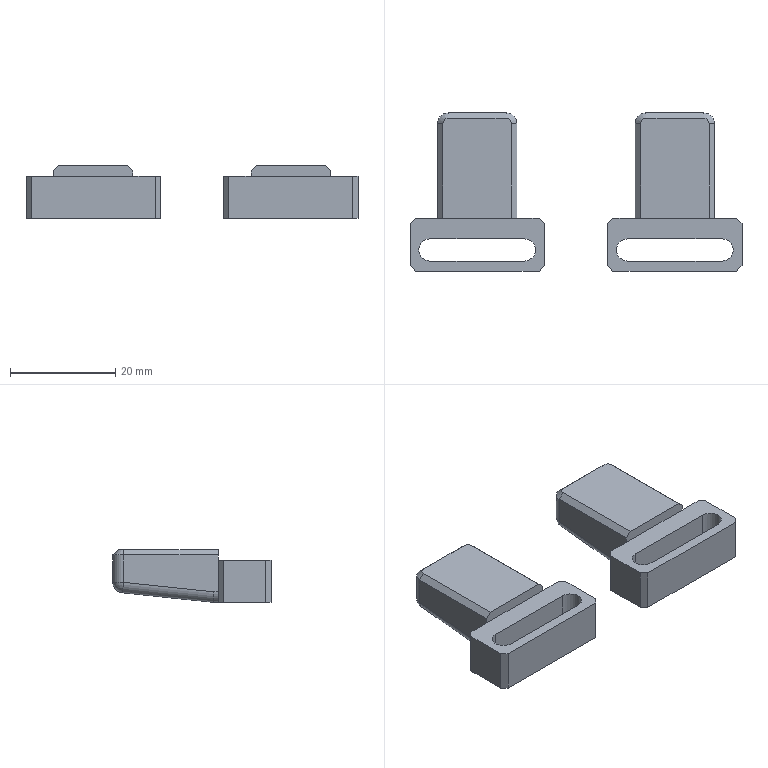NC program | NX | posted with a generic post | part box 63 x 30 x 10 mm
Lines 1610 to 2151 of 2151:
(ZLEVEL_PROFILE_COPY , TOOL : D3)
N3188 T17 M6
N3190 G54
N3192 G17 G0 G90 X-22.132 Y-11.6 B0. C0. S9500 M3
N3194 G43 Z30. H17
N3196 Z-0.5
N3198 G94 G1 X-9.558 Z-1.159 F1000.
N3200 X-9.23 Y-11.356 Z-1.18
N3202 X-9.121 Y-10.962 Z-1.202
N3204 X-9.26 Y-10.604 Z-1.222
N3206 X-9.558 Y-10.4 Z-1.241
N3208 X-27.942 Z-2.204
N3210 X-28.24 Y-10.604 Z-2.223
N3212 X-28.379 Y-10.962 Z-2.243
N3214 X-28.27 Y-11.356 Z-2.265
N3216 X-27.942 Y-11.6 Z-2.286
N3218 X-27.75 Z-2.296
N3220 X-9.75 F1200.
N3222 G3 X-9.15 Y-11. R0.6
N3224 X-9.75 Y-10.4 R0.6
N3226 G1 X-27.75
N3228 G3 X-28.35 Y-11. R0.6
N3230 X-27.75 Y-11.6 R0.6
N3232 G1 X-10.775 Z-2.593
N3234 X-9.75
N3236 G3 X-9.15 Y-11. R0.6
N3238 X-9.75 Y-10.4 R0.6
N3240 G1 X-27.75
N3242 G3 X-28.35 Y-11. R0.6
N3244 X-27.75 Y-11.6 R0.6
N3246 G1 X-10.775 Z-2.889
N3248 X-9.75
N3250 G3 X-9.15 Y-11. R0.6
N3252 X-9.75 Y-10.4 R0.6
N3254 G1 X-27.75
N3256 G3 X-28.35 Y-11. R0.6
N3258 X-27.75 Y-11.6 R0.6
N3260 G1 X-10.775 Z-3.185
N3262 X-9.75
N3264 G3 X-9.15 Y-11. R0.6
N3266 X-9.75 Y-10.4 R0.6
N3268 G1 X-27.75
N3270 G3 X-28.35 Y-11. R0.6
N3272 X-27.75 Y-11.6 R0.6
N3274 G1 X-10.775 Z-3.481
N3276 X-9.75
N3278 G3 X-9.15 Y-11. R0.6
N3280 X-9.75 Y-10.4 R0.6
N3282 G1 X-27.75
N3284 G3 X-28.35 Y-11. R0.6
N3286 X-27.75 Y-11.6 R0.6
N3288 G1 X-10.775 Z-3.778
N3290 X-9.75
N3292 G3 X-9.15 Y-11. R0.6
N3294 X-9.75 Y-10.4 R0.6
N3296 G1 X-27.75
N3298 G3 X-28.35 Y-11. R0.6
N3300 X-27.75 Y-11.6 R0.6
N3302 G1 X-10.775 Z-4.074
N3304 X-9.75
N3306 G3 X-9.15 Y-11. R0.6
N3308 X-9.75 Y-10.4 R0.6
N3310 G1 X-27.75
N3312 G3 X-28.35 Y-11. R0.6
N3314 X-27.75 Y-11.6 R0.6
N3316 G1 X-10.775 Z-4.37
N3318 X-9.75
N3320 G3 X-9.15 Y-11. R0.6
N3322 X-9.75 Y-10.4 R0.6
N3324 G1 X-27.75
N3326 G3 X-28.35 Y-11. R0.6
N3328 X-27.75 Y-11.6 R0.6
N3330 G1 X-10.775 Z-4.667
N3332 X-9.75
N3334 G3 X-9.15 Y-11. R0.6
N3336 X-9.75 Y-10.4 R0.6
N3338 G1 X-27.75
N3340 G3 X-28.35 Y-11. R0.6
N3342 X-27.75 Y-11.6 R0.6
N3344 G1 X-10.775 Z-4.963
N3346 X-9.75
N3348 G3 X-9.15 Y-11. R0.6
N3350 X-9.75 Y-10.4 R0.6
N3352 G1 X-27.75
N3354 G3 X-28.35 Y-11. R0.6
N3356 X-27.75 Y-11.6 R0.6
N3358 G1 X-10.775 Z-5.259
N3360 X-9.75
N3362 G3 X-9.15 Y-11. R0.6
N3364 X-9.75 Y-10.4 R0.6
N3366 G1 X-27.75
N3368 G3 X-28.35 Y-11. R0.6
N3370 X-27.75 Y-11.6 R0.6
N3372 G1 X-10.775 Z-5.556
N3374 X-9.75
N3376 G3 X-9.15 Y-11. R0.6
N3378 X-9.75 Y-10.4 R0.6
N3380 G1 X-27.75
N3382 G3 X-28.35 Y-11. R0.6
N3384 X-27.75 Y-11.6 R0.6
N3386 G1 X-10.775 Z-5.852
N3388 X-9.75
N3390 G3 X-9.15 Y-11. R0.6
N3392 X-9.75 Y-10.4 R0.6
N3394 G1 X-27.75
N3396 G3 X-28.35 Y-11. R0.6
N3398 X-27.75 Y-11.6 R0.6
N3400 G1 X-10.775 Z-6.148
N3402 X-9.75
N3404 G3 X-9.15 Y-11. R0.6
N3406 X-9.75 Y-10.4 R0.6
N3408 G1 X-27.75
N3410 G3 X-28.35 Y-11. R0.6
N3412 X-27.75 Y-11.6 R0.6
N3414 G1 X-10.775 Z-6.444
N3416 X-9.75
N3418 G3 X-9.15 Y-11. R0.6
N3420 X-9.75 Y-10.4 R0.6
N3422 G1 X-27.75
N3424 G3 X-28.35 Y-11. R0.6
N3426 X-27.75 Y-11.6 R0.6
N3428 G1 X-10.775 Z-6.741
N3430 X-9.75
N3432 G3 X-9.15 Y-11. R0.6
N3434 X-9.75 Y-10.4 R0.6
N3436 G1 X-27.75
N3438 G3 X-28.35 Y-11. R0.6
N3440 X-27.75 Y-11.6 R0.6
N3442 G1 X-10.775 Z-7.037
N3444 X-9.75
N3446 G3 X-9.15 Y-11. R0.6
N3448 X-9.75 Y-10.4 R0.6
N3450 G1 X-27.75
N3452 G3 X-28.35 Y-11. R0.6
N3454 X-27.75 Y-11.6 R0.6
N3456 G1 X-10.775 Z-7.333
N3458 X-9.75
N3460 G3 X-9.15 Y-11. R0.6
N3462 X-9.75 Y-10.4 R0.6
N3464 G1 X-27.75
N3466 G3 X-28.35 Y-11. R0.6
N3468 X-27.75 Y-11.6 R0.6
N3470 G1 X-10.775 Z-7.63
N3472 X-9.75
N3474 G3 X-9.15 Y-11. R0.6
N3476 X-9.75 Y-10.4 R0.6
N3478 G1 X-27.75
N3480 G3 X-28.35 Y-11. R0.6
N3482 X-27.75 Y-11.6 R0.6
N3484 G1 X-10.775 Z-7.926
N3486 X-9.75
N3488 G3 X-9.15 Y-11. R0.6
N3490 X-9.75 Y-10.4 R0.6
N3492 G1 X-27.75
N3494 G3 X-28.35 Y-11. R0.6
N3496 X-27.75 Y-11.6 R0.6
N3498 G1 X-10.775 Z-8.222
N3500 X-9.75
N3502 G3 X-9.15 Y-11. R0.6
N3504 X-9.75 Y-10.4 R0.6
N3506 G1 X-27.75
N3508 G3 X-28.35 Y-11. R0.6
N3510 X-27.75 Y-11.6 R0.6
N3512 G1 X-10.775 Z-8.519
N3514 X-9.75
N3516 G3 X-9.15 Y-11. R0.6
N3518 X-9.75 Y-10.4 R0.6
N3520 G1 X-27.75
N3522 G3 X-28.35 Y-11. R0.6
N3524 X-27.75 Y-11.6 R0.6
N3526 G1 X-10.775 Z-8.815
N3528 X-9.75
N3530 G3 X-9.15 Y-11. R0.6
N3532 X-9.75 Y-10.4 R0.6
N3534 G1 X-27.75
N3536 G3 X-28.35 Y-11. R0.6
N3538 X-27.75 Y-11.6 R0.6
N3540 G1 X-10.775 Z-9.111
N3542 X-9.75
N3544 G3 X-9.15 Y-11. R0.6
N3546 X-9.75 Y-10.4 R0.6
N3548 G1 X-27.75
N3550 G3 X-28.35 Y-11. R0.6
N3552 X-27.75 Y-11.6 R0.6
N3554 G1 X-10.775 Z-9.407
N3556 X-9.75
N3558 G3 X-9.15 Y-11. R0.6
N3560 X-9.75 Y-10.4 R0.6
N3562 G1 X-27.75
N3564 G3 X-28.35 Y-11. R0.6
N3566 X-27.75 Y-11.6 R0.6
N3568 G1 X-10.775 Z-9.704
N3570 X-9.75
N3572 G3 X-9.15 Y-11. R0.6
N3574 X-9.75 Y-10.4 R0.6
N3576 G1 X-27.75
N3578 G3 X-28.35 Y-11. R0.6
N3580 X-27.75 Y-11.6 R0.6
N3582 G1 X-10.775 Z-10.
N3584 X-9.75
N3586 G3 X-9.15 Y-11. R0.6
N3588 X-9.75 Y-10.4 R0.6
N3590 G1 X-27.75
N3592 G3 X-28.35 Y-11. R0.6
N3594 X-27.75 Y-11.6 R0.6
N3596 G1 X-10.775
N3598 Z-8.5
N3600 G0 Z30.
N3602 X15.368
N3604 Z-0.5
N3606 G1 X27.942 Z-1.159 F1000.
N3608 X28.27 Y-11.356 Z-1.18
N3610 X28.379 Y-10.962 Z-1.202
N3612 X28.24 Y-10.604 Z-1.222
N3614 X27.942 Y-10.4 Z-1.241
N3616 X9.558 Z-2.204
N3618 X9.26 Y-10.604 Z-2.223
N3620 X9.121 Y-10.962 Z-2.243
N3622 X9.23 Y-11.356 Z-2.265
N3624 X9.558 Y-11.6 Z-2.286
N3626 X9.75 Z-2.296
N3628 X27.75 F1200.
N3630 G3 X28.35 Y-11. R0.6
N3632 X27.75 Y-10.4 R0.6
N3634 G1 X9.75
N3636 G3 X9.15 Y-11. R0.6
N3638 X9.75 Y-11.6 R0.6
N3640 G1 X26.725 Z-2.593
N3642 X27.75
N3644 G3 X28.35 Y-11. R0.6
N3646 X27.75 Y-10.4 R0.6
N3648 G1 X9.75
N3650 G3 X9.15 Y-11. R0.6
N3652 X9.75 Y-11.6 R0.6
N3654 G1 X26.725 Z-2.889
N3656 X27.75
N3658 G3 X28.35 Y-11. R0.6
N3660 X27.75 Y-10.4 R0.6
N3662 G1 X9.75
N3664 G3 X9.15 Y-11. R0.6
N3666 X9.75 Y-11.6 R0.6
N3668 G1 X26.725 Z-3.185
N3670 X27.75
N3672 G3 X28.35 Y-11. R0.6
N3674 X27.75 Y-10.4 R0.6
N3676 G1 X9.75
N3678 G3 X9.15 Y-11. R0.6
N3680 X9.75 Y-11.6 R0.6
N3682 G1 X26.725 Z-3.481
N3684 X27.75
N3686 G3 X28.35 Y-11. R0.6
N3688 X27.75 Y-10.4 R0.6
N3690 G1 X9.75
N3692 G3 X9.15 Y-11. R0.6
N3694 X9.75 Y-11.6 R0.6
N3696 G1 X26.725 Z-3.778
N3698 X27.75
N3700 G3 X28.35 Y-11. R0.6
N3702 X27.75 Y-10.4 R0.6
N3704 G1 X9.75
N3706 G3 X9.15 Y-11. R0.6
N3708 X9.75 Y-11.6 R0.6
N3710 G1 X26.725 Z-4.074
N3712 X27.75
N3714 G3 X28.35 Y-11. R0.6
N3716 X27.75 Y-10.4 R0.6
N3718 G1 X9.75
N3720 G3 X9.15 Y-11. R0.6
N3722 X9.75 Y-11.6 R0.6
N3724 G1 X26.725 Z-4.37
N3726 X27.75
N3728 G3 X28.35 Y-11. R0.6
N3730 X27.75 Y-10.4 R0.6
N3732 G1 X9.75
N3734 G3 X9.15 Y-11. R0.6
N3736 X9.75 Y-11.6 R0.6
N3738 G1 X26.725 Z-4.667
N3740 X27.75
N3742 G3 X28.35 Y-11. R0.6
N3744 X27.75 Y-10.4 R0.6
N3746 G1 X9.75
N3748 G3 X9.15 Y-11. R0.6
N3750 X9.75 Y-11.6 R0.6
N3752 G1 X26.725 Z-4.963
N3754 X27.75
N3756 G3 X28.35 Y-11. R0.6
N3758 X27.75 Y-10.4 R0.6
N3760 G1 X9.75
N3762 G3 X9.15 Y-11. R0.6
N3764 X9.75 Y-11.6 R0.6
N3766 G1 X26.725 Z-5.259
N3768 X27.75
N3770 G3 X28.35 Y-11. R0.6
N3772 X27.75 Y-10.4 R0.6
N3774 G1 X9.75
N3776 G3 X9.15 Y-11. R0.6
N3778 X9.75 Y-11.6 R0.6
N3780 G1 X26.725 Z-5.556
N3782 X27.75
N3784 G3 X28.35 Y-11. R0.6
N3786 X27.75 Y-10.4 R0.6
N3788 G1 X9.75
N3790 G3 X9.15 Y-11. R0.6
N3792 X9.75 Y-11.6 R0.6
N3794 G1 X26.725 Z-5.852
N3796 X27.75
N3798 G3 X28.35 Y-11. R0.6
N3800 X27.75 Y-10.4 R0.6
N3802 G1 X9.75
N3804 G3 X9.15 Y-11. R0.6
N3806 X9.75 Y-11.6 R0.6
N3808 G1 X26.725 Z-6.148
N3810 X27.75
N3812 G3 X28.35 Y-11. R0.6
N3814 X27.75 Y-10.4 R0.6
N3816 G1 X9.75
N3818 G3 X9.15 Y-11. R0.6
N3820 X9.75 Y-11.6 R0.6
N3822 G1 X26.725 Z-6.444
N3824 X27.75
N3826 G3 X28.35 Y-11. R0.6
N3828 X27.75 Y-10.4 R0.6
N3830 G1 X9.75
N3832 G3 X9.15 Y-11. R0.6
N3834 X9.75 Y-11.6 R0.6
N3836 G1 X26.725 Z-6.741
N3838 X27.75
N3840 G3 X28.35 Y-11. R0.6
N3842 X27.75 Y-10.4 R0.6
N3844 G1 X9.75
N3846 G3 X9.15 Y-11. R0.6
N3848 X9.75 Y-11.6 R0.6
N3850 G1 X26.725 Z-7.037
N3852 X27.75
N3854 G3 X28.35 Y-11. R0.6
N3856 X27.75 Y-10.4 R0.6
N3858 G1 X9.75
N3860 G3 X9.15 Y-11. R0.6
N3862 X9.75 Y-11.6 R0.6
N3864 G1 X26.725 Z-7.333
N3866 X27.75
N3868 G3 X28.35 Y-11. R0.6
N3870 X27.75 Y-10.4 R0.6
N3872 G1 X9.75
N3874 G3 X9.15 Y-11. R0.6
N3876 X9.75 Y-11.6 R0.6
N3878 G1 X26.725 Z-7.63
N3880 X27.75
N3882 G3 X28.35 Y-11. R0.6
N3884 X27.75 Y-10.4 R0.6
N3886 G1 X9.75
N3888 G3 X9.15 Y-11. R0.6
N3890 X9.75 Y-11.6 R0.6
N3892 G1 X26.725 Z-7.926
N3894 X27.75
N3896 G3 X28.35 Y-11. R0.6
N3898 X27.75 Y-10.4 R0.6
N3900 G1 X9.75
N3902 G3 X9.15 Y-11. R0.6
N3904 X9.75 Y-11.6 R0.6
N3906 G1 X26.725 Z-8.222
N3908 X27.75
N3910 G3 X28.35 Y-11. R0.6
N3912 X27.75 Y-10.4 R0.6
N3914 G1 X9.75
N3916 G3 X9.15 Y-11. R0.6
N3918 X9.75 Y-11.6 R0.6
N3920 G1 X26.725 Z-8.519
N3922 X27.75
N3924 G3 X28.35 Y-11. R0.6
N3926 X27.75 Y-10.4 R0.6
N3928 G1 X9.75
N3930 G3 X9.15 Y-11. R0.6
N3932 X9.75 Y-11.6 R0.6
N3934 G1 X26.725 Z-8.815
N3936 X27.75
N3938 G3 X28.35 Y-11. R0.6
N3940 X27.75 Y-10.4 R0.6
N3942 G1 X9.75
N3944 G3 X9.15 Y-11. R0.6
N3946 X9.75 Y-11.6 R0.6
N3948 G1 X26.725 Z-9.111
N3950 X27.75
N3952 G3 X28.35 Y-11. R0.6
N3954 X27.75 Y-10.4 R0.6
N3956 G1 X9.75
N3958 G3 X9.15 Y-11. R0.6
N3960 X9.75 Y-11.6 R0.6
N3962 G1 X26.725 Z-9.407
N3964 X27.75
N3966 G3 X28.35 Y-11. R0.6
N3968 X27.75 Y-10.4 R0.6
N3970 G1 X9.75
N3972 G3 X9.15 Y-11. R0.6
N3974 X9.75 Y-11.6 R0.6
N3976 G1 X26.725 Z-9.704
N3978 X27.75
N3980 G3 X28.35 Y-11. R0.6
N3982 X27.75 Y-10.4 R0.6
N3984 G1 X9.75
N3986 G3 X9.15 Y-11. R0.6
N3988 X9.75 Y-11.6 R0.6
N3990 G1 X26.725 Z-10.
N3992 X27.75
N3994 G3 X28.35 Y-11. R0.6
N3996 X27.75 Y-10.4 R0.6
N3998 G1 X9.75
N4000 G3 X9.15 Y-11. R0.6
N4002 X9.75 Y-11.6 R0.6
N4004 G1 X26.725
N4006 Z-8.5
N4008 G0 Z30.
N4010 M5
(PLANAR_MILL_COPY_COPY_COPY_COPY_COPY_COPY_1_COPY_1 , TOOL : D6A45)
N4012 T01 M6
N4014 G54
N4016 G17 G0 G90 X-27.45 Y3.134 B0. C0. S9500 M3
N4018 G43 Z30. H1
N4020 Z-0.2
N4022 G94 G1 Z-1.7 F1250.
N4024 G3 X-26.95 Y4. R1.
N4026 G1 Y13.
N4028 G2 X-24.25 Y15.7 R2.7
N4030 G1 X-13.25
N4032 G2 X-10.55 Y13. R2.7
N4034 G1 Y-5.
N4036 G2 X-12.25 Y-6.7 R1.7
N4038 G1 X-25.25
N4040 G2 X-26.95 Y-5. R1.7
N4042 G1 Y4.
N4044 G3 X-27.45 Y4.866 R1.
N4046 G1 Z-0.2
N4048 G0 Z30.
N4050 X27.45
N4052 Z-0.2
N4054 G1 Z-1.7
N4056 G3 X26.95 Y4. R1.
N4058 G1 Y-5.
N4060 G2 X25.25 Y-6.7 R1.7
N4062 G1 X12.25
N4064 G2 X10.55 Y-5. R1.7
N4066 G1 Y13.
N4068 G2 X13.25 Y15.7 R2.7
N4070 G1 X24.25
N4072 G2 X26.95 Y13. R2.7
N4074 G1 Y4.
N4076 G3 X27.45 Y3.134 R1.
N4078 G1 Z-0.2
N4080 G0 Z30.
(PLANAR_MILL_COPY_COPY_COPY_COPY_COPY_COPY_1_COPY_1_COPY , TOOL : D6A45)
N4082 X-20.02 Y-11.
N4084 Z-1.5
N4086 G1 Z-3.
N4088 X-19.616 Y-11.7
N4090 G3 X-18.75 Y-12.2 R1.
N4092 G1 X-9.75
N4094 G3 X-8.55 Y-11. R1.2
N4096 X-9.75 Y-9.8 R1.2
N4098 G1 X-27.75
N4100 G3 X-28.95 Y-11. R1.2
N4102 X-27.75 Y-12.2 R1.2
N4104 G1 X-18.75
N4106 G3 X-17.884 Y-11.7 R1.
N4108 G1 X-17.48 Y-11.
N4110 Z-1.5
N4112 G0 Z30.
N4114 X-6.55 Y-2.83
N4116 Z-1.5
N4118 G1 Z-3.
N4120 X-7.25 Y-3.234
N4122 G3 X-7.75 Y-4.1 R1.
N4124 G1 X-7.041
N4126 G2 X-6.334 Y-4.393 R1.
N4128 G1 X-5.393 Y-5.334
N4130 G2 X-5.1 Y-6.041 R1.
N4132 G1 Y-13.959
N4134 G2 X-5.393 Y-14.666 R1.
N4136 G1 X-6.334 Y-15.607
N4138 G2 X-7.041 Y-15.9 R1.
N4140 G1 X-30.459
N4142 G2 X-31.166 Y-15.607 R1.
N4144 G1 X-32.107 Y-14.666
N4146 G2 X-32.4 Y-13.959 R1.
N4148 G1 Y-6.041
N4150 G2 X-32.107 Y-5.334 R1.
N4152 G1 X-31.166 Y-4.393
N4154 G2 X-30.459 Y-4.1 R1.
N4156 G1 X-29.75
N4158 G3 X-30.25 Y-3.234 R1.
N4160 G1 X-30.95 Y-2.83
N4162 Z-1.5
N4164 G0 Z30.
N4166 X30.95
N4168 Z-1.5
N4170 G1 Z-3.
N4172 X30.25 Y-3.234
N4174 G3 X29.75 Y-4.1 R1.
N4176 G1 X30.459
N4178 G2 X31.166 Y-4.393 R1.
N4180 G1 X32.107 Y-5.334
N4182 G2 X32.4 Y-6.041 R1.
N4184 G1 Y-13.959
N4186 G2 X32.107 Y-14.666 R1.
N4188 G1 X31.166 Y-15.607
N4190 G2 X30.459 Y-15.9 R1.
N4192 G1 X7.041
N4194 G2 X6.334 Y-15.607 R1.
N4196 G1 X5.393 Y-14.666
N4198 G2 X5.1 Y-13.959 R1.
N4200 G1 Y-6.041
N4202 G2 X5.393 Y-5.334 R1.
N4204 G1 X6.334 Y-4.393
N4206 G2 X7.041 Y-4.1 R1.
N4208 G1 X7.75
N4210 G3 X7.25 Y-3.234 R1.
N4212 G1 X6.55 Y-2.83
N4214 Z-1.5
N4216 G0 Z30.
N4218 X17.48 Y-11.
N4220 Z-1.5
N4222 G1 Z-3.
N4224 X17.884 Y-11.7
N4226 G3 X18.75 Y-12.2 R1.
N4228 G1 X27.75
N4230 G3 X28.95 Y-11. R1.2
N4232 X27.75 Y-9.8 R1.2
N4234 G1 X9.75
N4236 G3 X8.55 Y-11. R1.2
N4238 X9.75 Y-12.2 R1.2
N4240 G1 X18.75
N4242 G3 X19.616 Y-11.7 R1.
N4244 G1 X20.02 Y-11.
N4246 Z-1.5
N4248 G0 Z30.
N4250 M5
N4252 M2